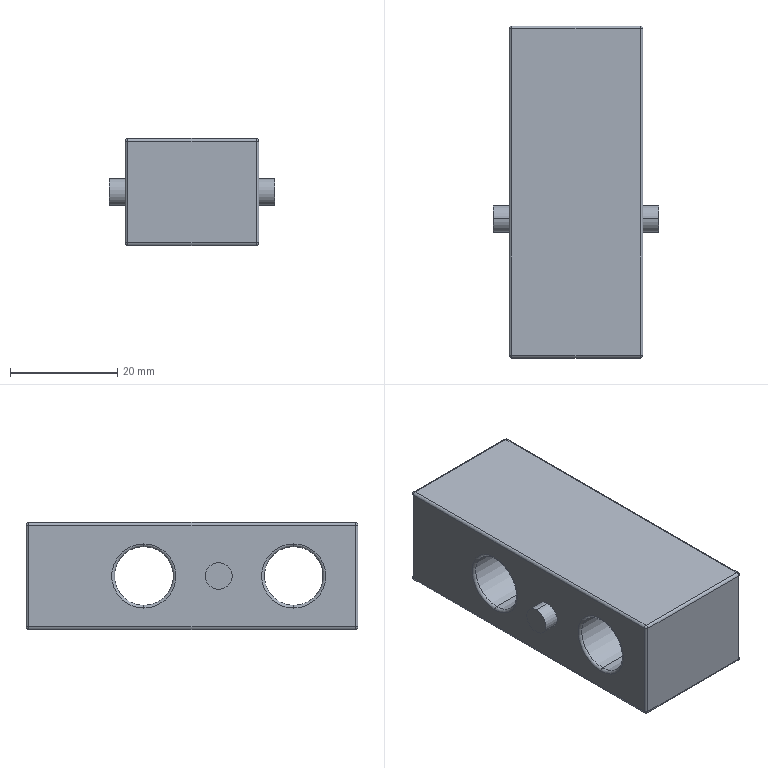Part | SolidWorks | features ICE 2, Extrusion 1, Fillet 1 | 1 solid | 49 faces | box 31 x 62 x 20 mm | volume 24637 mm3 | cylinder 22 | torus 10 | plane 9 | sphere 8 | commonest cylinder face diameters 1 x12 5 x4 11 x4 12 x2
STEP:
#1=CARTESIAN_POINT('',(12.5,-5.,-2.5));
#2=VERTEX_POINT('',#1);
#3=CARTESIAN_POINT('',(12.5,-5.,2.5));
#4=VERTEX_POINT('',#3);
#5=CARTESIAN_POINT('',(12.5,-5.,0.));
#6=DIRECTION('',(1.,0.,0.));
#7=DIRECTION('',(0.,0.,-1.));
#8=AXIS2_PLACEMENT_3D('',#5,#6,#7);
#9=CIRCLE('',#8,2.5);
#10=EDGE_CURVE('',#2,#4,#9,.T.);
#11=ORIENTED_EDGE('',*,*,#10,.T.);
#12=CARTESIAN_POINT('',(15.5,-5.,2.5));
#13=VERTEX_POINT('',#12);
#14=CARTESIAN_POINT('',(-25.571,-5.,2.5));
#15=DIRECTION('',(1.,0.,0.));
#16=VECTOR('',#15,1000.);
#17=LINE('',#14,#16);
#18=EDGE_CURVE('',#4,#13,#17,.T.);
#19=ORIENTED_EDGE('',*,*,#18,.T.);
#20=CARTESIAN_POINT('',(15.5,-5.,-2.5));
#21=VERTEX_POINT('',#20);
#22=CARTESIAN_POINT('',(15.5,-5.,0.));
#23=DIRECTION('',(1.,0.,0.));
#24=DIRECTION('',(0.,0.,-1.));
#25=AXIS2_PLACEMENT_3D('',#22,#23,#24);
#26=CIRCLE('',#25,2.5);
#27=EDGE_CURVE('',#21,#13,#26,.T.);
#28=ORIENTED_EDGE('',*,*,#27,.F.);
#29=CARTESIAN_POINT('',(-25.571,-5.,-2.5));
#30=DIRECTION('',(1.,0.,0.));
#31=VECTOR('',#30,1000.);
#32=LINE('',#29,#31);
#33=EDGE_CURVE('',#2,#21,#32,.T.);
#34=ORIENTED_EDGE('',*,*,#33,.F.);
#35=EDGE_LOOP('',(#11,#19,#28,#34));
#36=FACE_OUTER_BOUND('',#35,.T.);
#37=CARTESIAN_POINT('',(-25.571,-5.,0.));
#38=DIRECTION('',(1.,0.,0.));
#39=DIRECTION('',(0.,0.,-1.));
#40=AXIS2_PLACEMENT_3D('',#37,#38,#39);
#41=CYLINDRICAL_SURFACE('',#40,2.5);
#42=ADVANCED_FACE('',(#36),#41,.T.);
#43=CARTESIAN_POINT('',(-15.5,-5.,2.5));
#44=VERTEX_POINT('',#43);
#45=CARTESIAN_POINT('',(-15.5,-5.,-2.5));
#46=VERTEX_POINT('',#45);
#47=CARTESIAN_POINT('',(-15.5,-5.,0.));
#48=DIRECTION('',(-1.,0.,0.));
#49=DIRECTION('',(0.,0.,-1.));
#50=AXIS2_PLACEMENT_3D('',#47,#48,#49);
#51=CIRCLE('',#50,2.5);
#52=EDGE_CURVE('',#44,#46,#51,.T.);
#53=ORIENTED_EDGE('',*,*,#52,.F.);
#54=CARTESIAN_POINT('',(-12.5,-5.,2.5));
#55=VERTEX_POINT('',#54);
#56=CARTESIAN_POINT('',(-25.571,-5.,2.5));
#57=DIRECTION('',(1.,0.,0.));
#58=VECTOR('',#57,1000.);
#59=LINE('',#56,#58);
#60=EDGE_CURVE('',#44,#55,#59,.T.);
#61=ORIENTED_EDGE('',*,*,#60,.T.);
#62=CARTESIAN_POINT('',(-12.5,-5.,-2.5));
#63=VERTEX_POINT('',#62);
#64=CARTESIAN_POINT('',(-12.5,-5.,0.));
#65=DIRECTION('',(1.,0.,0.));
#66=DIRECTION('',(0.,0.,-1.));
#67=AXIS2_PLACEMENT_3D('',#64,#65,#66);
#68=CIRCLE('',#67,2.5);
#69=EDGE_CURVE('',#63,#55,#68,.T.);
#70=ORIENTED_EDGE('',*,*,#69,.F.);
#71=CARTESIAN_POINT('',(-25.571,-5.,-2.5));
#72=DIRECTION('',(1.,0.,0.));
#73=VECTOR('',#72,1000.);
#74=LINE('',#71,#73);
#75=EDGE_CURVE('',#46,#63,#74,.T.);
#76=ORIENTED_EDGE('',*,*,#75,.F.);
#77=EDGE_LOOP('',(#53,#61,#70,#76));
#78=FACE_OUTER_BOUND('',#77,.T.);
#79=CARTESIAN_POINT('',(-25.571,-5.,0.));
#80=DIRECTION('',(1.,0.,0.));
#81=DIRECTION('',(0.,0.,-1.));
#82=AXIS2_PLACEMENT_3D('',#79,#80,#81);
#83=CYLINDRICAL_SURFACE('',#82,2.5);
#84=ADVANCED_FACE('',(#78),#83,.T.);
#85=CARTESIAN_POINT('',(12.5,-19.,6.));
#86=VERTEX_POINT('',#85);
#87=CARTESIAN_POINT('',(12.5,-19.,-6.));
#88=VERTEX_POINT('',#87);
#89=CARTESIAN_POINT('',(12.5,-19.,0.));
#90=DIRECTION('',(-1.,0.,0.));
#91=DIRECTION('',(0.,0.,-1.));
#92=AXIS2_PLACEMENT_3D('',#89,#90,#91);
#93=CIRCLE('',#92,6.);
#94=EDGE_CURVE('',#86,#88,#93,.T.);
#95=ORIENTED_EDGE('',*,*,#94,.F.);
#96=CARTESIAN_POINT('',(12.,-19.,5.5));
#97=VERTEX_POINT('',#96);
#98=CARTESIAN_POINT('',(12.,-19.,6.));
#99=DIRECTION('',(0.,1.,0.));
#100=DIRECTION('',(0.,0.,1.));
#101=AXIS2_PLACEMENT_3D('',#98,#99,#100);
#102=CIRCLE('',#101,0.5);
#103=EDGE_CURVE('',#86,#97,#102,.T.);
#104=ORIENTED_EDGE('',*,*,#103,.T.);
#105=CARTESIAN_POINT('',(12.,-19.,-5.5));
#106=VERTEX_POINT('',#105);
#107=CARTESIAN_POINT('',(12.,-19.,0.));
#108=DIRECTION('',(1.,0.,0.));
#109=DIRECTION('',(0.,0.,-1.));
#110=AXIS2_PLACEMENT_3D('',#107,#108,#109);
#111=CIRCLE('',#110,5.5);
#112=EDGE_CURVE('',#106,#97,#111,.T.);
#113=ORIENTED_EDGE('',*,*,#112,.F.);
#114=CARTESIAN_POINT('',(12.,-19.,-6.));
#115=DIRECTION('',(0.,-1.,0.));
#116=DIRECTION('',(0.,0.,-1.));
#117=AXIS2_PLACEMENT_3D('',#114,#115,#116);
#118=CIRCLE('',#117,0.5);
#119=EDGE_CURVE('',#88,#106,#118,.T.);
#120=ORIENTED_EDGE('',*,*,#119,.F.);
#121=EDGE_LOOP('',(#95,#104,#113,#120));
#122=FACE_OUTER_BOUND('',#121,.T.);
#123=CARTESIAN_POINT('',(12.,-19.,0.));
#124=DIRECTION('',(1.,0.,0.));
#125=DIRECTION('',(0.,0.,-1.));
#126=AXIS2_PLACEMENT_3D('',#123,#124,#125);
#127=TOROIDAL_SURFACE('',#126,6.,0.5);
#128=ADVANCED_FACE('',(#122),#127,.T.);
#129=CARTESIAN_POINT('',(12.5,9.,6.));
#130=VERTEX_POINT('',#129);
#131=CARTESIAN_POINT('',(12.5,9.,-6.));
#132=VERTEX_POINT('',#131);
#133=CARTESIAN_POINT('',(12.5,9.,0.));
#134=DIRECTION('',(-1.,0.,0.));
#135=DIRECTION('',(0.,0.,-1.));
#136=AXIS2_PLACEMENT_3D('',#133,#134,#135);
#137=CIRCLE('',#136,6.);
#138=EDGE_CURVE('',#130,#132,#137,.T.);
#139=ORIENTED_EDGE('',*,*,#138,.F.);
#140=CARTESIAN_POINT('',(12.,9.,5.5));
#141=VERTEX_POINT('',#140);
#142=CARTESIAN_POINT('',(12.,9.,6.));
#143=DIRECTION('',(0.,1.,0.));
#144=DIRECTION('',(0.,0.,1.));
#145=AXIS2_PLACEMENT_3D('',#142,#143,#144);
#146=CIRCLE('',#145,0.5);
#147=EDGE_CURVE('',#130,#141,#146,.T.);
#148=ORIENTED_EDGE('',*,*,#147,.T.);
#149=CARTESIAN_POINT('',(12.,9.,-5.5));
#150=VERTEX_POINT('',#149);
#151=CARTESIAN_POINT('',(12.,9.,0.));
#152=DIRECTION('',(1.,0.,0.));
#153=DIRECTION('',(0.,0.,-1.));
#154=AXIS2_PLACEMENT_3D('',#151,#152,#153);
#155=CIRCLE('',#154,5.5);
#156=EDGE_CURVE('',#150,#141,#155,.T.);
#157=ORIENTED_EDGE('',*,*,#156,.F.);
#158=CARTESIAN_POINT('',(12.,9.,-6.));
#159=DIRECTION('',(0.,-1.,0.));
#160=DIRECTION('',(0.,0.,-1.));
#161=AXIS2_PLACEMENT_3D('',#158,#159,#160);
#162=CIRCLE('',#161,0.5);
#163=EDGE_CURVE('',#132,#150,#162,.T.);
#164=ORIENTED_EDGE('',*,*,#163,.F.);
#165=EDGE_LOOP('',(#139,#148,#157,#164));
#166=FACE_OUTER_BOUND('',#165,.T.);
#167=CARTESIAN_POINT('',(12.,9.,0.));
#168=DIRECTION('',(1.,0.,0.));
#169=DIRECTION('',(0.,0.,-1.));
#170=AXIS2_PLACEMENT_3D('',#167,#168,#169);
#171=TOROIDAL_SURFACE('',#170,6.,0.5);
#172=ADVANCED_FACE('',(#166),#171,.T.);
#173=CARTESIAN_POINT('',(-6.,24.,-9.5));
#174=VERTEX_POINT('',#173);
#175=CARTESIAN_POINT('',(6.,24.,-9.5));
#176=VERTEX_POINT('',#175);
#177=CARTESIAN_POINT('',(0.,24.,-9.5));
#178=DIRECTION('',(0.,0.,-1.));
#179=DIRECTION('',(1.,0.,0.));
#180=AXIS2_PLACEMENT_3D('',#177,#178,#179);
#181=CIRCLE('',#180,6.);
#182=EDGE_CURVE('',#174,#176,#181,.T.);
#183=ORIENTED_EDGE('',*,*,#182,.F.);
#184=CARTESIAN_POINT('',(-6.5,24.,-10.));
#185=VERTEX_POINT('',#184);
#186=CARTESIAN_POINT('',(-6.5,24.,-9.5));
#187=DIRECTION('',(0.,1.,0.));
#188=DIRECTION('',(-1.,0.,0.));
#189=AXIS2_PLACEMENT_3D('',#186,#187,#188);
#190=CIRCLE('',#189,0.5);
#191=EDGE_CURVE('',#174,#185,#190,.T.);
#192=ORIENTED_EDGE('',*,*,#191,.T.);
#193=CARTESIAN_POINT('',(0.,30.5,-10.));
#194=VERTEX_POINT('',#193);
#195=CARTESIAN_POINT('',(0.,24.,-10.));
#196=DIRECTION('',(0.,0.,1.));
#197=DIRECTION('',(1.,0.,0.));
#198=AXIS2_PLACEMENT_3D('',#195,#196,#197);
#199=CIRCLE('',#198,6.5);
#200=EDGE_CURVE('',#194,#185,#199,.T.);
#201=ORIENTED_EDGE('',*,*,#200,.F.);
#202=CARTESIAN_POINT('',(6.5,24.,-10.));
#203=VERTEX_POINT('',#202);
#204=CARTESIAN_POINT('',(0.,24.,-10.));
#205=DIRECTION('',(0.,0.,1.));
#206=DIRECTION('',(1.,0.,0.));
#207=AXIS2_PLACEMENT_3D('',#204,#205,#206);
#208=CIRCLE('',#207,6.5);
#209=EDGE_CURVE('',#203,#194,#208,.T.);
#210=ORIENTED_EDGE('',*,*,#209,.F.);
#211=CARTESIAN_POINT('',(6.5,24.,-9.5));
#212=DIRECTION('',(0.,-1.,0.));
#213=DIRECTION('',(0.,0.,-1.));
#214=AXIS2_PLACEMENT_3D('',#211,#212,#213);
#215=CIRCLE('',#214,0.5);
#216=EDGE_CURVE('',#176,#203,#215,.T.);
#217=ORIENTED_EDGE('',*,*,#216,.F.);
#218=EDGE_LOOP('',(#183,#192,#201,#210,#217));
#219=FACE_OUTER_BOUND('',#218,.T.);
#220=CARTESIAN_POINT('',(0.,24.,-9.5));
#221=DIRECTION('',(0.,0.,1.));
#222=DIRECTION('',(1.,0.,0.));
#223=AXIS2_PLACEMENT_3D('',#220,#221,#222);
#224=TOROIDAL_SURFACE('',#223,6.5,0.5);
#225=ADVANCED_FACE('',(#219),#224,.T.);
#226=CARTESIAN_POINT('',(-12.,-19.,5.5));
#227=VERTEX_POINT('',#226);
#228=CARTESIAN_POINT('',(-12.,-19.,-5.5));
#229=VERTEX_POINT('',#228);
#230=CARTESIAN_POINT('',(-12.,-19.,0.));
#231=DIRECTION('',(-1.,0.,0.));
#232=DIRECTION('',(0.,0.,-1.));
#233=AXIS2_PLACEMENT_3D('',#230,#231,#232);
#234=CIRCLE('',#233,5.5);
#235=EDGE_CURVE('',#227,#229,#234,.T.);
#236=ORIENTED_EDGE('',*,*,#235,.F.);
#237=CARTESIAN_POINT('',(-12.5,-19.,6.));
#238=VERTEX_POINT('',#237);
#239=CARTESIAN_POINT('',(-12.,-19.,6.));
#240=DIRECTION('',(0.,1.,0.));
#241=DIRECTION('',(0.,0.,1.));
#242=AXIS2_PLACEMENT_3D('',#239,#240,#241);
#243=CIRCLE('',#242,0.5);
#244=EDGE_CURVE('',#227,#238,#243,.T.);
#245=ORIENTED_EDGE('',*,*,#244,.T.);
#246=CARTESIAN_POINT('',(-12.5,-19.,-6.));
#247=VERTEX_POINT('',#246);
#248=CARTESIAN_POINT('',(-12.5,-19.,0.));
#249=DIRECTION('',(1.,0.,0.));
#250=DIRECTION('',(0.,0.,-1.));
#251=AXIS2_PLACEMENT_3D('',#248,#249,#250);
#252=CIRCLE('',#251,6.);
#253=EDGE_CURVE('',#247,#238,#252,.T.);
#254=ORIENTED_EDGE('',*,*,#253,.F.);
#255=CARTESIAN_POINT('',(-12.,-19.,-6.));
#256=DIRECTION('',(0.,-1.,0.));
#257=DIRECTION('',(0.,0.,-1.));
#258=AXIS2_PLACEMENT_3D('',#255,#256,#257);
#259=CIRCLE('',#258,0.5);
#260=EDGE_CURVE('',#229,#247,#259,.T.);
#261=ORIENTED_EDGE('',*,*,#260,.F.);
#262=EDGE_LOOP('',(#236,#245,#254,#261));
#263=FACE_OUTER_BOUND('',#262,.T.);
#264=CARTESIAN_POINT('',(-12.,-19.,0.));
#265=DIRECTION('',(1.,0.,0.));
#266=DIRECTION('',(0.,0.,-1.));
#267=AXIS2_PLACEMENT_3D('',#264,#265,#266);
#268=TOROIDAL_SURFACE('',#267,6.,0.5);
#269=ADVANCED_FACE('',(#263),#268,.T.);
#270=CARTESIAN_POINT('',(-12.,9.,5.5));
#271=VERTEX_POINT('',#270);
#272=CARTESIAN_POINT('',(-12.,9.,-5.5));
#273=VERTEX_POINT('',#272);
#274=CARTESIAN_POINT('',(-12.,9.,0.));
#275=DIRECTION('',(-1.,0.,0.));
#276=DIRECTION('',(0.,0.,-1.));
#277=AXIS2_PLACEMENT_3D('',#274,#275,#276);
#278=CIRCLE('',#277,5.5);
#279=EDGE_CURVE('',#271,#273,#278,.T.);
#280=ORIENTED_EDGE('',*,*,#279,.F.);
#281=CARTESIAN_POINT('',(-12.5,9.,6.));
#282=VERTEX_POINT('',#281);
#283=CARTESIAN_POINT('',(-12.,9.,6.));
#284=DIRECTION('',(0.,1.,0.));
#285=DIRECTION('',(0.,0.,1.));
#286=AXIS2_PLACEMENT_3D('',#283,#284,#285);
#287=CIRCLE('',#286,0.5);
#288=EDGE_CURVE('',#271,#282,#287,.T.);
#289=ORIENTED_EDGE('',*,*,#288,.T.);
#290=CARTESIAN_POINT('',(-12.5,9.,-6.));
#291=VERTEX_POINT('',#290);
#292=CARTESIAN_POINT('',(-12.5,9.,0.));
#293=DIRECTION('',(1.,0.,0.));
#294=DIRECTION('',(0.,0.,-1.));
#295=AXIS2_PLACEMENT_3D('',#292,#293,#294);
#296=CIRCLE('',#295,6.);
#297=EDGE_CURVE('',#291,#282,#296,.T.);
#298=ORIENTED_EDGE('',*,*,#297,.F.);
#299=CARTESIAN_POINT('',(-12.,9.,-6.));
#300=DIRECTION('',(0.,-1.,0.));
#301=DIRECTION('',(0.,0.,-1.));
#302=AXIS2_PLACEMENT_3D('',#299,#300,#301);
#303=CIRCLE('',#302,0.5);
#304=EDGE_CURVE('',#273,#291,#303,.T.);
#305=ORIENTED_EDGE('',*,*,#304,.F.);
#306=EDGE_LOOP('',(#280,#289,#298,#305));
#307=FACE_OUTER_BOUND('',#306,.T.);
#308=CARTESIAN_POINT('',(-12.,9.,0.));
#309=DIRECTION('',(1.,0.,0.));
#310=DIRECTION('',(0.,0.,-1.));
#311=AXIS2_PLACEMENT_3D('',#308,#309,#310);
#312=TOROIDAL_SURFACE('',#311,6.,0.5);
#313=ADVANCED_FACE('',(#307),#312,.T.);
#314=CARTESIAN_POINT('',(6.,24.,5.));
#315=VERTEX_POINT('',#314);
#316=CARTESIAN_POINT('',(-6.,24.,5.));
#317=VERTEX_POINT('',#316);
#318=CARTESIAN_POINT('',(0.,24.,5.));
#319=DIRECTION('',(0.,0.,-1.));
#320=DIRECTION('',(-1.,0.,0.));
#321=AXIS2_PLACEMENT_3D('',#318,#319,#320);
#322=CIRCLE('',#321,6.);
#323=EDGE_CURVE('',#315,#317,#322,.T.);
#324=ORIENTED_EDGE('',*,*,#323,.F.);
#325=CARTESIAN_POINT('',(6.,24.,5.));
#326=DIRECTION('',(0.,0.,-1.));
#327=VECTOR('',#326,1000.);
#328=LINE('',#325,#327);
#329=EDGE_CURVE('',#315,#176,#328,.T.);
#330=ORIENTED_EDGE('',*,*,#329,.T.);
#331=CARTESIAN_POINT('',(0.,24.,-9.5));
#332=DIRECTION('',(0.,0.,-1.));
#333=DIRECTION('',(1.,0.,0.));
#334=AXIS2_PLACEMENT_3D('',#331,#332,#333);
#335=CIRCLE('',#334,6.);
#336=EDGE_CURVE('',#176,#174,#335,.T.);
#337=ORIENTED_EDGE('',*,*,#336,.T.);
#338=CARTESIAN_POINT('',(-6.,24.,5.));
#339=DIRECTION('',(0.,0.,-1.));
#340=VECTOR('',#339,1000.);
#341=LINE('',#338,#340);
#342=EDGE_CURVE('',#317,#174,#341,.T.);
#343=ORIENTED_EDGE('',*,*,#342,.F.);
#344=EDGE_LOOP('',(#324,#330,#337,#343));
#345=FACE_OUTER_BOUND('',#344,.T.);
#346=CARTESIAN_POINT('',(0.,24.,5.));
#347=DIRECTION('',(0.,0.,-1.));
#348=DIRECTION('',(-1.,0.,0.));
#349=AXIS2_PLACEMENT_3D('',#346,#347,#348);
#350=CYLINDRICAL_SURFACE('',#349,6.);
#351=ADVANCED_FACE('',(#345),#350,.F.);
#352=CARTESIAN_POINT('',(12.,9.,0.));
#353=DIRECTION('',(1.,0.,0.));
#354=DIRECTION('',(0.,0.,-1.));
#355=AXIS2_PLACEMENT_3D('',#352,#353,#354);
#356=CIRCLE('',#355,5.5);
#357=EDGE_CURVE('',#141,#150,#356,.T.);
#358=ORIENTED_EDGE('',*,*,#357,.T.);
#359=CARTESIAN_POINT('',(12.5,9.,-5.5));
#360=DIRECTION('',(-1.,0.,0.));
#361=VECTOR('',#360,1000.);
#362=LINE('',#359,#361);
#363=EDGE_CURVE('',#150,#273,#362,.T.);
#364=ORIENTED_EDGE('',*,*,#363,.T.);
#365=CARTESIAN_POINT('',(-12.,9.,0.));
#366=DIRECTION('',(-1.,0.,0.));
#367=DIRECTION('',(0.,0.,-1.));
#368=AXIS2_PLACEMENT_3D('',#365,#366,#367);
#369=CIRCLE('',#368,5.5);
#370=EDGE_CURVE('',#273,#271,#369,.T.);
#371=ORIENTED_EDGE('',*,*,#370,.T.);
#372=CARTESIAN_POINT('',(12.5,9.,5.5));
#373=DIRECTION('',(-1.,0.,0.));
#374=VECTOR('',#373,1000.);
#375=LINE('',#372,#374);
#376=EDGE_CURVE('',#141,#271,#375,.T.);
#377=ORIENTED_EDGE('',*,*,#376,.F.);
#378=EDGE_LOOP('',(#358,#364,#371,#377));
#379=FACE_OUTER_BOUND('',#378,.T.);
#380=CARTESIAN_POINT('',(12.5,9.,0.));
#381=DIRECTION('',(-1.,0.,0.));
#382=DIRECTION('',(0.,0.,1.));
#383=AXIS2_PLACEMENT_3D('',#380,#381,#382);
#384=CYLINDRICAL_SURFACE('',#383,5.5);
#385=ADVANCED_FACE('',(#379),#384,.F.);
#386=CARTESIAN_POINT('',(12.,-19.,0.));
#387=DIRECTION('',(1.,0.,0.));
#388=DIRECTION('',(0.,0.,-1.));
#389=AXIS2_PLACEMENT_3D('',#386,#387,#388);
#390=CIRCLE('',#389,5.5);
#391=EDGE_CURVE('',#97,#106,#390,.T.);
#392=ORIENTED_EDGE('',*,*,#391,.T.);
#393=CARTESIAN_POINT('',(12.5,-19.,-5.5));
#394=DIRECTION('',(-1.,0.,0.));
#395=VECTOR('',#394,1000.);
#396=LINE('',#393,#395);
#397=EDGE_CURVE('',#106,#229,#396,.T.);
#398=ORIENTED_EDGE('',*,*,#397,.T.);
#399=CARTESIAN_POINT('',(-12.,-19.,0.));
#400=DIRECTION('',(-1.,0.,0.));
#401=DIRECTION('',(0.,0.,-1.));
#402=AXIS2_PLACEMENT_3D('',#399,#400,#401);
#403=CIRCLE('',#402,5.5);
#404=EDGE_CURVE('',#229,#227,#403,.T.);
#405=ORIENTED_EDGE('',*,*,#404,.T.);
#406=CARTESIAN_POINT('',(12.5,-19.,5.5));
#407=DIRECTION('',(-1.,0.,0.));
#408=VECTOR('',#407,1000.);
#409=LINE('',#406,#408);
#410=EDGE_CURVE('',#97,#227,#409,.T.);
#411=ORIENTED_EDGE('',*,*,#410,.F.);
#412=EDGE_LOOP('',(#392,#398,#405,#411));
#413=FACE_OUTER_BOUND('',#412,.T.);
#414=CARTESIAN_POINT('',(12.5,-19.,0.));
#415=DIRECTION('',(-1.,0.,0.));
#416=DIRECTION('',(0.,0.,1.));
#417=AXIS2_PLACEMENT_3D('',#414,#415,#416);
#418=CYLINDRICAL_SURFACE('',#417,5.5);
#419=ADVANCED_FACE('',(#413),#418,.F.);
#420=ORIENTED_EDGE('',*,*,#10,.F.);
#421=CARTESIAN_POINT('',(12.5,-5.,0.));
#422=DIRECTION('',(1.,0.,0.));
#423=DIRECTION('',(0.,0.,-1.));
#424=AXIS2_PLACEMENT_3D('',#421,#422,#423);
#425=CIRCLE('',#424,2.5);
#426=EDGE_CURVE('',#4,#2,#425,.T.);
#427=ORIENTED_EDGE('',*,*,#426,.F.);
#428=EDGE_LOOP('',(#420,#427));
#429=FACE_BOUND('',#428,.T.);
#430=CARTESIAN_POINT('',(12.5,9.,0.));
#431=DIRECTION('',(-1.,0.,0.));
#432=DIRECTION('',(0.,0.,-1.));
#433=AXIS2_PLACEMENT_3D('',#430,#431,#432);
#434=CIRCLE('',#433,6.);
#435=EDGE_CURVE('',#132,#130,#434,.T.);
#436=ORIENTED_EDGE('',*,*,#435,.T.);
#437=ORIENTED_EDGE('',*,*,#138,.T.);
#438=EDGE_LOOP('',(#436,#437));
#439=FACE_BOUND('',#438,.T.);
#440=CARTESIAN_POINT('',(12.5,-19.,0.));
#441=DIRECTION('',(-1.,0.,0.));
#442=DIRECTION('',(0.,0.,-1.));
#443=AXIS2_PLACEMENT_3D('',#440,#441,#442);
#444=CIRCLE('',#443,6.);
#445=EDGE_CURVE('',#88,#86,#444,.T.);
#446=ORIENTED_EDGE('',*,*,#445,.T.);
#447=ORIENTED_EDGE('',*,*,#94,.T.);
#448=EDGE_LOOP('',(#446,#447));
#449=FACE_BOUND('',#448,.T.);
#450=CARTESIAN_POINT('',(12.5,-30.5,9.5));
#451=VERTEX_POINT('',#450);
#452=CARTESIAN_POINT('',(12.5,-30.5,-9.5));
#453=VERTEX_POINT('',#452);
#454=CARTESIAN_POINT('',(12.5,-30.5,-10.));
#455=DIRECTION('',(0.,0.,-1.));
#456=VECTOR('',#455,1000.);
#457=LINE('',#454,#456);
#458=EDGE_CURVE('',#451,#453,#457,.T.);
#459=ORIENTED_EDGE('',*,*,#458,.T.);
#460=CARTESIAN_POINT('',(12.5,30.5,-9.5));
#461=VERTEX_POINT('',#460);
#462=CARTESIAN_POINT('',(12.5,31.,-9.5));
#463=DIRECTION('',(0.,1.,0.));
#464=VECTOR('',#463,1000.);
#465=LINE('',#462,#464);
#466=EDGE_CURVE('',#453,#461,#465,.T.);
#467=ORIENTED_EDGE('',*,*,#466,.T.);
#468=CARTESIAN_POINT('',(12.5,30.5,9.5));
#469=VERTEX_POINT('',#468);
#470=CARTESIAN_POINT('',(12.5,30.5,10.));
#471=DIRECTION('',(0.,0.,1.));
#472=VECTOR('',#471,1000.);
#473=LINE('',#470,#472);
#474=EDGE_CURVE('',#461,#469,#473,.T.);
#475=ORIENTED_EDGE('',*,*,#474,.T.);
#476=CARTESIAN_POINT('',(12.5,-31.,9.5));
#477=DIRECTION('',(0.,-1.,0.));
#478=VECTOR('',#477,1000.);
#479=LINE('',#476,#478);
#480=EDGE_CURVE('',#469,#451,#479,.T.);
#481=ORIENTED_EDGE('',*,*,#480,.T.);
#482=EDGE_LOOP('',(#459,#467,#475,#481));
#483=FACE_OUTER_BOUND('',#482,.T.);
#484=CARTESIAN_POINT('',(12.5,0.,0.));
#485=DIRECTION('',(1.,0.,0.));
#486=DIRECTION('',(0.,0.,-1.));
#487=AXIS2_PLACEMENT_3D('',#484,#485,#486);
#488=PLANE('',#487);
#489=ADVANCED_FACE('',(#429,#439,#449,#483),#488,.T.);
#490=ORIENTED_EDGE('',*,*,#69,.T.);
#491=CARTESIAN_POINT('',(-12.5,-5.,0.));
#492=DIRECTION('',(1.,0.,0.));
#493=DIRECTION('',(0.,0.,-1.));
#494=AXIS2_PLACEMENT_3D('',#491,#492,#493);
#495=CIRCLE('',#494,2.5);
#496=EDGE_CURVE('',#55,#63,#495,.T.);
#497=ORIENTED_EDGE('',*,*,#496,.T.);
#498=EDGE_LOOP('',(#490,#497));
#499=FACE_BOUND('',#498,.T.);
#500=ORIENTED_EDGE('',*,*,#297,.T.);
#501=CARTESIAN_POINT('',(-12.5,9.,0.));
#502=DIRECTION('',(1.,0.,0.));
#503=DIRECTION('',(0.,0.,-1.));
#504=AXIS2_PLACEMENT_3D('',#501,#502,#503);
#505=CIRCLE('',#504,6.);
#506=EDGE_CURVE('',#282,#291,#505,.T.);
#507=ORIENTED_EDGE('',*,*,#506,.T.);
#508=EDGE_LOOP('',(#500,#507));
#509=FACE_BOUND('',#508,.T.);
#510=ORIENTED_EDGE('',*,*,#253,.T.);
#511=CARTESIAN_POINT('',(-12.5,-19.,0.));
#512=DIRECTION('',(1.,0.,0.));
#513=DIRECTION('',(0.,0.,-1.));
#514=AXIS2_PLACEMENT_3D('',#511,#512,#513);
#515=CIRCLE('',#514,6.);
#516=EDGE_CURVE('',#238,#247,#515,.T.);
#517=ORIENTED_EDGE('',*,*,#516,.T.);
#518=EDGE_LOOP('',(#510,#517));
#519=FACE_BOUND('',#518,.T.);
#520=CARTESIAN_POINT('',(-12.5,30.5,-9.5));
#521=VERTEX_POINT('',#520);
#522=CARTESIAN_POINT('',(-12.5,-30.5,-9.5));
#523=VERTEX_POINT('',#522);
#524=CARTESIAN_POINT('',(-12.5,0.,-9.5));
#525=DIRECTION('',(0.,-1.,0.));
#526=VECTOR('',#525,1000.);
#527=LINE('',#524,#526);
#528=EDGE_CURVE('',#521,#523,#527,.T.);
#529=ORIENTED_EDGE('',*,*,#528,.T.);
#530=CARTESIAN_POINT('',(-12.5,-30.5,9.5));
#531=VERTEX_POINT('',#530);
#532=CARTESIAN_POINT('',(-12.5,-30.5,0.));
#533=DIRECTION('',(0.,0.,1.));
#534=VECTOR('',#533,1000.);
#535=LINE('',#532,#534);
#536=EDGE_CURVE('',#523,#531,#535,.T.);
#537=ORIENTED_EDGE('',*,*,#536,.T.);
#538=CARTESIAN_POINT('',(-12.5,30.5,9.5));
#539=VERTEX_POINT('',#538);
#540=CARTESIAN_POINT('',(-12.5,0.,9.5));
#541=DIRECTION('',(0.,1.,0.));
#542=VECTOR('',#541,1000.);
#543=LINE('',#540,#542);
#544=EDGE_CURVE('',#531,#539,#543,.T.);
#545=ORIENTED_EDGE('',*,*,#544,.T.);
#546=CARTESIAN_POINT('',(-12.5,30.5,0.));
#547=DIRECTION('',(0.,0.,-1.));
#548=VECTOR('',#547,1000.);
#549=LINE('',#546,#548);
#550=EDGE_CURVE('',#539,#521,#549,.T.);
#551=ORIENTED_EDGE('',*,*,#550,.T.);
#552=EDGE_LOOP('',(#529,#537,#545,#551));
#553=FACE_OUTER_BOUND('',#552,.T.);
#554=CARTESIAN_POINT('',(-12.5,0.,0.));
#555=DIRECTION('',(1.,0.,0.));
#556=DIRECTION('',(0.,0.,-1.));
#557=AXIS2_PLACEMENT_3D('',#554,#555,#556);
#558=PLANE('',#557);
#559=ADVANCED_FACE('',(#499,#509,#519,#553),#558,.F.);
#560=CARTESIAN_POINT('',(-12.,30.5,10.));
#561=VERTEX_POINT('',#560);
#562=CARTESIAN_POINT('',(-12.,-30.5,10.));
#563=VERTEX_POINT('',#562);
#564=CARTESIAN_POINT('',(-12.,-31.,10.));
#565=DIRECTION('',(0.,-1.,0.));
#566=VECTOR('',#565,1000.);
#567=LINE('',#564,#566);
#568=EDGE_CURVE('',#561,#563,#567,.T.);
#569=ORIENTED_EDGE('',*,*,#568,.T.);
#570=CARTESIAN_POINT('',(12.,-30.5,10.));
#571=VERTEX_POINT('',#570);
#572=CARTESIAN_POINT('',(12.5,-30.5,10.));
#573=DIRECTION('',(1.,0.,0.));
#574=VECTOR('',#573,1000.);
#575=LINE('',#572,#574);
#576=EDGE_CURVE('',#563,#571,#575,.T.);
#577=ORIENTED_EDGE('',*,*,#576,.T.);
#578=CARTESIAN_POINT('',(12.,30.5,10.));
#579=VERTEX_POINT('',#578);
#580=CARTESIAN_POINT('',(12.,31.,10.));
#581=DIRECTION('',(0.,1.,0.));
#582=VECTOR('',#581,1000.);
#583=LINE('',#580,#582);
#584=EDGE_CURVE('',#571,#579,#583,.T.);
#585=ORIENTED_EDGE('',*,*,#584,.T.);
#586=CARTESIAN_POINT('',(12.5,30.5,10.));
#587=DIRECTION('',(-1.,0.,0.));
#588=VECTOR('',#587,1000.);
#589=LINE('',#586,#588);
#590=EDGE_CURVE('',#579,#561,#589,.T.);
#591=ORIENTED_EDGE('',*,*,#590,.T.);
#592=EDGE_LOOP('',(#569,#577,#585,#591));
#593=FACE_OUTER_BOUND('',#592,.T.);
#594=CARTESIAN_POINT('',(12.5,-31.,10.));
#595=DIRECTION('',(0.,0.,-1.));
#596=DIRECTION('',(-1.,0.,0.));
#597=AXIS2_PLACEMENT_3D('',#594,#595,#596);
#598=PLANE('',#597);
#599=ADVANCED_FACE('',(#593),#598,.F.);
#600=CARTESIAN_POINT('',(12.,-31.,-9.5));
#601=VERTEX_POINT('',#600);
#602=CARTESIAN_POINT('',(12.,-31.,9.5));
#603=VERTEX_POINT('',#602);
#604=CARTESIAN_POINT('',(12.,-31.,10.));
#605=DIRECTION('',(0.,0.,1.));
#606=VECTOR('',#605,1000.);
#607=LINE('',#604,#606);
#608=EDGE_CURVE('',#601,#603,#607,.T.);
#609=ORIENTED_EDGE('',*,*,#608,.T.);
#610=CARTESIAN_POINT('',(-12.,-31.,9.5));
#611=VERTEX_POINT('',#610);
#612=CARTESIAN_POINT('',(12.5,-31.,9.5));
#613=DIRECTION('',(-1.,0.,0.));
#614=VECTOR('',#613,1000.);
#615=LINE('',#612,#614);
#616=EDGE_CURVE('',#603,#611,#615,.T.);
#617=ORIENTED_EDGE('',*,*,#616,.T.);
#618=CARTESIAN_POINT('',(-12.,-31.,-9.5));
#619=VERTEX_POINT('',#618);
#620=CARTESIAN_POINT('',(-12.,-31.,-10.));
#621=DIRECTION('',(0.,0.,-1.));
#622=VECTOR('',#621,1000.);
#623=LINE('',#620,#622);
#624=EDGE_CURVE('',#611,#619,#623,.T.);
#625=ORIENTED_EDGE('',*,*,#624,.T.);
#626=CARTESIAN_POINT('',(12.5,-31.,-9.5));
#627=DIRECTION('',(1.,0.,0.));
#628=VECTOR('',#627,1000.);
#629=LINE('',#626,#628);
#630=EDGE_CURVE('',#619,#601,#629,.T.);
#631=ORIENTED_EDGE('',*,*,#630,.T.);
#632=EDGE_LOOP('',(#609,#617,#625,#631));
#633=FACE_OUTER_BOUND('',#632,.T.);
#634=CARTESIAN_POINT('',(12.5,-31.,-10.));
#635=DIRECTION('',(0.,1.,0.));
#636=DIRECTION('',(0.,0.,1.));
#637=AXIS2_PLACEMENT_3D('',#634,#635,#636);
#638=PLANE('',#637);
#639=ADVANCED_FACE('',(#633),#638,.F.);
#640=ORIENTED_EDGE('',*,*,#200,.T.);
#641=CARTESIAN_POINT('',(0.,24.,-10.));
#642=DIRECTION('',(0.,0.,1.));
#643=DIRECTION('',(1.,0.,0.));
#644=AXIS2_PLACEMENT_3D('',#641,#642,#643);
#645=CIRCLE('',#644,6.5);
#646=EDGE_CURVE('',#185,#203,#645,.T.);
#647=ORIENTED_EDGE('',*,*,#646,.T.);
#648=ORIENTED_EDGE('',*,*,#209,.T.);
#649=CARTESIAN_POINT('',(12.,30.5,-10.));
#650=VERTEX_POINT('',#649);
#651=CARTESIAN_POINT('',(12.5,30.5,-10.));
#652=DIRECTION('',(1.,0.,0.));
#653=VECTOR('',#652,1000.);
#654=LINE('',#651,#653);
#655=EDGE_CURVE('',#194,#650,#654,.T.);
#656=ORIENTED_EDGE('',*,*,#655,.T.);
#657=CARTESIAN_POINT('',(12.,-30.5,-10.));
#658=VERTEX_POINT('',#657);
#659=CARTESIAN_POINT('',(12.,-31.,-10.));
#660=DIRECTION('',(0.,-1.,0.));
#661=VECTOR('',#660,1000.);
#662=LINE('',#659,#661);
#663=EDGE_CURVE('',#650,#658,#662,.T.);
#664=ORIENTED_EDGE('',*,*,#663,.T.);
#665=CARTESIAN_POINT('',(-12.,-30.5,-10.));
#666=VERTEX_POINT('',#665);
#667=CARTESIAN_POINT('',(12.5,-30.5,-10.));
#668=DIRECTION('',(-1.,0.,0.));
#669=VECTOR('',#668,1000.);
#670=LINE('',#667,#669);
#671=EDGE_CURVE('',#658,#666,#670,.T.);
#672=ORIENTED_EDGE('',*,*,#671,.T.);
#673=CARTESIAN_POINT('',(-12.,30.5,-10.));
#674=VERTEX_POINT('',#673);
#675=CARTESIAN_POINT('',(-12.,-31.,-10.));
#676=DIRECTION('',(0.,1.,0.));
#677=VECTOR('',#676,1000.);
#678=LINE('',#675,#677);
#679=EDGE_CURVE('',#666,#674,#678,.T.);
#680=ORIENTED_EDGE('',*,*,#679,.T.);
#681=CARTESIAN_POINT('',(12.5,30.5,-10.));
#682=DIRECTION('',(1.,0.,0.));
#683=VECTOR('',#682,1000.);
#684=LINE('',#681,#683);
#685=EDGE_CURVE('',#674,#194,#684,.T.);
#686=ORIENTED_EDGE('',*,*,#685,.T.);
#687=EDGE_LOOP('',(#640,#647,#648,#656,#664,#672,#680,#686));
#688=FACE_OUTER_BOUND('',#687,.T.);
#689=CARTESIAN_POINT('',(12.5,-31.,-10.));
#690=DIRECTION('',(0.,0.,1.));
#691=DIRECTION('',(1.,0.,0.));
#692=AXIS2_PLACEMENT_3D('',#689,#690,#691);
#693=PLANE('',#692);
#694=ADVANCED_FACE('',(#688),#693,.F.);
#695=CARTESIAN_POINT('',(12.,31.,9.5));
#696=VERTEX_POINT('',#695);
#697=CARTESIAN_POINT('',(12.,31.,-9.5));
#698=VERTEX_POINT('',#697);
#699=CARTESIAN_POINT('',(12.,31.,-10.));
#700=DIRECTION('',(0.,0.,-1.));
#701=VECTOR('',#700,1000.);
#702=LINE('',#699,#701);
#703=EDGE_CURVE('',#696,#698,#702,.T.);
#704=ORIENTED_EDGE('',*,*,#703,.T.);
#705=CARTESIAN_POINT('',(-12.,31.,-9.5));
#706=VERTEX_POINT('',#705);
#707=CARTESIAN_POINT('',(12.5,31.,-9.5));
#708=DIRECTION('',(-1.,0.,0.));
#709=VECTOR('',#708,1000.);
#710=LINE('',#707,#709);
#711=EDGE_CURVE('',#698,#706,#710,.T.);
#712=ORIENTED_EDGE('',*,*,#711,.T.);
#713=CARTESIAN_POINT('',(-12.,31.,9.5));
#714=VERTEX_POINT('',#713);
#715=CARTESIAN_POINT('',(-12.,31.,-10.));
#716=DIRECTION('',(0.,0.,1.));
#717=VECTOR('',#716,1000.);
#718=LINE('',#715,#717);
#719=EDGE_CURVE('',#706,#714,#718,.T.);
#720=ORIENTED_EDGE('',*,*,#719,.T.);
#721=CARTESIAN_POINT('',(12.5,31.,9.5));
#722=DIRECTION('',(1.,0.,0.));
#723=VECTOR('',#722,1000.);
#724=LINE('',#721,#723);
#725=EDGE_CURVE('',#714,#696,#724,.T.);
#726=ORIENTED_EDGE('',*,*,#725,.T.);
#727=EDGE_LOOP('',(#704,#712,#720,#726));
#728=FACE_OUTER_BOUND('',#727,.T.);
#729=CARTESIAN_POINT('',(12.5,31.,-10.));
#730=DIRECTION('',(0.,-1.,0.));
#731=DIRECTION('',(0.,0.,-1.));
#732=AXIS2_PLACEMENT_3D('',#729,#730,#731);
#733=PLANE('',#732);
#734=ADVANCED_FACE('',(#728),#733,.F.);
#735=ORIENTED_EDGE('',*,*,#397,.F.);
#736=ORIENTED_EDGE('',*,*,#112,.T.);
#737=ORIENTED_EDGE('',*,*,#410,.T.);
#738=ORIENTED_EDGE('',*,*,#235,.T.);
#739=EDGE_LOOP('',(#735,#736,#737,#738));
#740=FACE_OUTER_BOUND('',#739,.T.);
#741=CARTESIAN_POINT('',(12.5,-19.,0.));
#742=DIRECTION('',(-1.,0.,0.));
#743=DIRECTION('',(0.,0.,1.));
#744=AXIS2_PLACEMENT_3D('',#741,#742,#743);
#745=CYLINDRICAL_SURFACE('',#744,5.5);
#746=ADVANCED_FACE('',(#740),#745,.F.);
#747=ORIENTED_EDGE('',*,*,#363,.F.);
#748=ORIENTED_EDGE('',*,*,#156,.T.);
#749=ORIENTED_EDGE('',*,*,#376,.T.);
#750=ORIENTED_EDGE('',*,*,#279,.T.);
#751=EDGE_LOOP('',(#747,#748,#749,#750));
#752=FACE_OUTER_BOUND('',#751,.T.);
#753=CARTESIAN_POINT('',(12.5,9.,0.));
#754=DIRECTION('',(-1.,0.,0.));
#755=DIRECTION('',(0.,0.,1.));
#756=AXIS2_PLACEMENT_3D('',#753,#754,#755);
#757=CYLINDRICAL_SURFACE('',#756,5.5);
#758=ADVANCED_FACE('',(#752),#757,.F.);
#759=ORIENTED_EDGE('',*,*,#329,.F.);
#760=CARTESIAN_POINT('',(0.,24.,5.));
#761=DIRECTION('',(0.,0.,-1.));
#762=DIRECTION('',(-1.,0.,0.));
#763=AXIS2_PLACEMENT_3D('',#760,#761,#762);
#764=CIRCLE('',#763,6.);
#765=EDGE_CURVE('',#317,#315,#764,.T.);
#766=ORIENTED_EDGE('',*,*,#765,.F.);
#767=ORIENTED_EDGE('',*,*,#342,.T.);
#768=ORIENTED_EDGE('',*,*,#182,.T.);
#769=EDGE_LOOP('',(#759,#766,#767,#768));
#770=FACE_OUTER_BOUND('',#769,.T.);
#771=CARTESIAN_POINT('',(0.,24.,5.));
#772=DIRECTION('',(0.,0.,-1.));
#773=DIRECTION('',(-1.,0.,0.));
#774=AXIS2_PLACEMENT_3D('',#771,#772,#773);
#775=CYLINDRICAL_SURFACE('',#774,6.);
#776=ADVANCED_FACE('',(#770),#775,.F.);
#777=ORIENTED_EDGE('',*,*,#765,.T.);
#778=ORIENTED_EDGE('',*,*,#323,.T.);
#779=EDGE_LOOP('',(#777,#778));
#780=FACE_OUTER_BOUND('',#779,.T.);
#781=CARTESIAN_POINT('',(0.,24.,5.));
#782=DIRECTION('',(0.,0.,-1.));
#783=DIRECTION('',(-1.,0.,0.));
#784=AXIS2_PLACEMENT_3D('',#781,#782,#783);
#785=PLANE('',#784);
#786=ADVANCED_FACE('',(#780),#785,.T.);
#787=CARTESIAN_POINT('',(12.,30.5,-9.5));
#788=DIRECTION('',(1.,0.,0.));
#789=DIRECTION('',(0.,0.,-1.));
#790=AXIS2_PLACEMENT_3D('',#787,#788,#789);
#791=CIRCLE('',#790,0.5);
#792=EDGE_CURVE('',#650,#698,#791,.T.);
#793=ORIENTED_EDGE('',*,*,#792,.F.);
#794=ORIENTED_EDGE('',*,*,#655,.F.);
#795=ORIENTED_EDGE('',*,*,#685,.F.);
#796=CARTESIAN_POINT('',(-12.,30.5,-9.5));
#797=DIRECTION('',(-1.,0.,0.));
#798=DIRECTION('',(0.,0.,1.));
#799=AXIS2_PLACEMENT_3D('',#796,#797,#798);
#800=CIRCLE('',#799,0.5);
#801=EDGE_CURVE('',#706,#674,#800,.T.);
#802=ORIENTED_EDGE('',*,*,#801,.F.);
#803=ORIENTED_EDGE('',*,*,#711,.F.);
#804=EDGE_LOOP('',(#793,#794,#795,#802,#803));
#805=FACE_OUTER_BOUND('',#804,.T.);
#806=CARTESIAN_POINT('',(12.5,30.5,-9.5));
#807=DIRECTION('',(-1.,0.,0.));
#808=DIRECTION('',(0.,0.,1.));
#809=AXIS2_PLACEMENT_3D('',#806,#807,#808);
#810=CYLINDRICAL_SURFACE('',#809,0.5);
#811=ADVANCED_FACE('',(#805),#810,.T.);
#812=CARTESIAN_POINT('',(12.,30.5,-9.5));
#813=DIRECTION('',(0.,-1.,0.));
#814=DIRECTION('',(0.,0.,1.));
#815=AXIS2_PLACEMENT_3D('',#812,#813,#814);
#816=CIRCLE('',#815,0.5);
#817=EDGE_CURVE('',#650,#461,#816,.T.);
#818=ORIENTED_EDGE('',*,*,#817,.F.);
#819=ORIENTED_EDGE('',*,*,#792,.T.);
#820=CARTESIAN_POINT('',(12.,30.5,-9.5));
#821=DIRECTION('',(0.,0.,1.));
#822=DIRECTION('',(-1.,0.,0.));
#823=AXIS2_PLACEMENT_3D('',#820,#821,#822);
#824=CIRCLE('',#823,0.5);
#825=EDGE_CURVE('',#461,#698,#824,.T.);
#826=ORIENTED_EDGE('',*,*,#825,.F.);
#827=EDGE_LOOP('',(#818,#819,#826));
#828=FACE_OUTER_BOUND('',#827,.T.);
#829=CARTESIAN_POINT('',(12.,30.5,-9.5));
#830=DIRECTION('',(0.,1.,0.));
#831=DIRECTION('',(1.,0.,0.));
#832=AXIS2_PLACEMENT_3D('',#829,#830,#831);
#833=SPHERICAL_SURFACE('',#832,0.5);
#834=ADVANCED_FACE('',(#828),#833,.T.);
#835=CARTESIAN_POINT('',(-12.,30.5,-9.5));
#836=DIRECTION('',(0.,0.,1.));
#837=DIRECTION('',(-1.,0.,0.));
#838=AXIS2_PLACEMENT_3D('',#835,#836,#837);
#839=CIRCLE('',#838,0.5);
#840=EDGE_CURVE('',#706,#521,#839,.T.);
#841=ORIENTED_EDGE('',*,*,#840,.F.);
#842=ORIENTED_EDGE('',*,*,#801,.T.);
#843=CARTESIAN_POINT('',(-12.,30.5,-9.5));
#844=DIRECTION('',(0.,-1.,0.));
#845=DIRECTION('',(0.,0.,1.));
#846=AXIS2_PLACEMENT_3D('',#843,#844,#845);
#847=CIRCLE('',#846,0.5);
#848=EDGE_CURVE('',#521,#674,#847,.T.);
#849=ORIENTED_EDGE('',*,*,#848,.F.);
#850=EDGE_LOOP('',(#841,#842,#849));
#851=FACE_OUTER_BOUND('',#850,.T.);
#852=CARTESIAN_POINT('',(-12.,30.5,-9.5));
#853=DIRECTION('',(0.,1.,0.));
#854=DIRECTION('',(1.,0.,0.));
#855=AXIS2_PLACEMENT_3D('',#852,#853,#854);
#856=SPHERICAL_SURFACE('',#855,0.5);
#857=ADVANCED_FACE('',(#851),#856,.T.);
#858=ORIENTED_EDGE('',*,*,#825,.T.);
#859=ORIENTED_EDGE('',*,*,#703,.F.);
#860=CARTESIAN_POINT('',(12.,30.5,9.5));
#861=DIRECTION('',(0.,0.,1.));
#862=DIRECTION('',(1.,0.,0.));
#863=AXIS2_PLACEMENT_3D('',#860,#861,#862);
#864=CIRCLE('',#863,0.5);
#865=EDGE_CURVE('',#469,#696,#864,.T.);
#866=ORIENTED_EDGE('',*,*,#865,.F.);
#867=ORIENTED_EDGE('',*,*,#474,.F.);
#868=EDGE_LOOP('',(#858,#859,#866,#867));
#869=FACE_OUTER_BOUND('',#868,.T.);
#870=CARTESIAN_POINT('',(12.,30.5,0.));
#871=DIRECTION('',(0.,0.,-1.));
#872=DIRECTION('',(-1.,0.,0.));
#873=AXIS2_PLACEMENT_3D('',#870,#871,#872);
#874=CYLINDRICAL_SURFACE('',#873,0.5);
#875=ADVANCED_FACE('',(#869),#874,.T.);
#876=ORIENTED_EDGE('',*,*,#817,.T.);
#877=ORIENTED_EDGE('',*,*,#466,.F.);
#878=CARTESIAN_POINT('',(12.,-30.5,-9.5));
#879=DIRECTION('',(0.,-1.,0.));
#880=DIRECTION('',(0.,0.,-1.));
#881=AXIS2_PLACEMENT_3D('',#878,#879,#880);
#882=CIRCLE('',#881,0.5);
#883=EDGE_CURVE('',#658,#453,#882,.T.);
#884=ORIENTED_EDGE('',*,*,#883,.F.);
#885=ORIENTED_EDGE('',*,*,#663,.F.);
#886=EDGE_LOOP('',(#876,#877,#884,#885));
#887=FACE_OUTER_BOUND('',#886,.T.);
#888=CARTESIAN_POINT('',(12.,0.,-9.5));
#889=DIRECTION('',(0.,-1.,0.));
#890=DIRECTION('',(0.,0.,-1.));
#891=AXIS2_PLACEMENT_3D('',#888,#889,#890);
#892=CYLINDRICAL_SURFACE('',#891,0.5);
#893=ADVANCED_FACE('',(#887),#892,.T.);
#894=CARTESIAN_POINT('',(-12.,-30.5,-9.5));
#895=DIRECTION('',(-1.,0.,0.));
#896=DIRECTION('',(0.,0.,1.));
#897=AXIS2_PLACEMENT_3D('',#894,#895,#896);
#898=CIRCLE('',#897,0.5);
#899=EDGE_CURVE('',#666,#619,#898,.T.);
#900=ORIENTED_EDGE('',*,*,#899,.F.);
#901=ORIENTED_EDGE('',*,*,#671,.F.);
#902=CARTESIAN_POINT('',(12.,-30.5,-9.5));
#903=DIRECTION('',(1.,0.,0.));
#904=DIRECTION('',(0.,0.,-1.));
#905=AXIS2_PLACEMENT_3D('',#902,#903,#904);
#906=CIRCLE('',#905,0.5);
#907=EDGE_CURVE('',#601,#658,#906,.T.);
#908=ORIENTED_EDGE('',*,*,#907,.F.);
#909=ORIENTED_EDGE('',*,*,#630,.F.);
#910=EDGE_LOOP('',(#900,#901,#908,#909));
#911=FACE_OUTER_BOUND('',#910,.T.);
#912=CARTESIAN_POINT('',(12.5,-30.5,-9.5));
#913=DIRECTION('',(-1.,0.,0.));
#914=DIRECTION('',(0.,0.,1.));
#915=AXIS2_PLACEMENT_3D('',#912,#913,#914);
#916=CYLINDRICAL_SURFACE('',#915,0.5);
#917=ADVANCED_FACE('',(#911),#916,.T.);
#918=ORIENTED_EDGE('',*,*,#848,.T.);
#919=ORIENTED_EDGE('',*,*,#679,.F.);
#920=CARTESIAN_POINT('',(-12.,-30.5,-9.5));
#921=DIRECTION('',(0.,-1.,0.));
#922=DIRECTION('',(0.,0.,-1.));
#923=AXIS2_PLACEMENT_3D('',#920,#921,#922);
#924=CIRCLE('',#923,0.5);
#925=EDGE_CURVE('',#523,#666,#924,.T.);
#926=ORIENTED_EDGE('',*,*,#925,.F.);
#927=ORIENTED_EDGE('',*,*,#528,.F.);
#928=EDGE_LOOP('',(#918,#919,#926,#927));
#929=FACE_OUTER_BOUND('',#928,.T.);
#930=CARTESIAN_POINT('',(-12.,-31.,-9.5));
#931=DIRECTION('',(0.,1.,0.));
#932=DIRECTION('',(0.,0.,1.));
#933=AXIS2_PLACEMENT_3D('',#930,#931,#932);
#934=CYLINDRICAL_SURFACE('',#933,0.5);
#935=ADVANCED_FACE('',(#929),#934,.T.);
#936=ORIENTED_EDGE('',*,*,#840,.T.);
#937=ORIENTED_EDGE('',*,*,#550,.F.);
#938=CARTESIAN_POINT('',(-12.,30.5,9.5));
#939=DIRECTION('',(0.,0.,1.));
#940=DIRECTION('',(1.,0.,0.));
#941=AXIS2_PLACEMENT_3D('',#938,#939,#940);
#942=CIRCLE('',#941,0.5);
#943=EDGE_CURVE('',#714,#539,#942,.T.);
#944=ORIENTED_EDGE('',*,*,#943,.F.);
#945=ORIENTED_EDGE('',*,*,#719,.F.);
#946=EDGE_LOOP('',(#936,#937,#944,#945));
#947=FACE_OUTER_BOUND('',#946,.T.);
#948=CARTESIAN_POINT('',(-12.,30.5,-10.));
#949=DIRECTION('',(0.,0.,1.));
#950=DIRECTION('',(1.,0.,0.));
#951=AXIS2_PLACEMENT_3D('',#948,#949,#950);
#952=CYLINDRICAL_SURFACE('',#951,0.5);
#953=ADVANCED_FACE('',(#947),#952,.T.);
#954=CARTESIAN_POINT('',(12.,30.5,9.5));
#955=DIRECTION('',(1.,0.,0.));
#956=DIRECTION('',(0.,0.,-1.));
#957=AXIS2_PLACEMENT_3D('',#954,#955,#956);
#958=CIRCLE('',#957,0.5);
#959=EDGE_CURVE('',#696,#579,#958,.T.);
#960=ORIENTED_EDGE('',*,*,#959,.F.);
#961=ORIENTED_EDGE('',*,*,#725,.F.);
#962=CARTESIAN_POINT('',(-12.,30.5,9.5));
#963=DIRECTION('',(-1.,0.,0.));
#964=DIRECTION('',(0.,0.,1.));
#965=AXIS2_PLACEMENT_3D('',#962,#963,#964);
#966=CIRCLE('',#965,0.5);
#967=EDGE_CURVE('',#561,#714,#966,.T.);
#968=ORIENTED_EDGE('',*,*,#967,.F.);
#969=ORIENTED_EDGE('',*,*,#590,.F.);
#970=EDGE_LOOP('',(#960,#961,#968,#969));
#971=FACE_OUTER_BOUND('',#970,.T.);
#972=CARTESIAN_POINT('',(12.5,30.5,9.5));
#973=DIRECTION('',(-1.,0.,0.));
#974=DIRECTION('',(0.,0.,1.));
#975=AXIS2_PLACEMENT_3D('',#972,#973,#974);
#976=CYLINDRICAL_SURFACE('',#975,0.5);
#977=ADVANCED_FACE('',(#971),#976,.T.);
#978=ORIENTED_EDGE('',*,*,#865,.T.);
#979=ORIENTED_EDGE('',*,*,#959,.T.);
#980=CARTESIAN_POINT('',(12.,30.5,9.5));
#981=DIRECTION('',(0.,-1.,0.));
#982=DIRECTION('',(0.,0.,1.));
#983=AXIS2_PLACEMENT_3D('',#980,#981,#982);
#984=CIRCLE('',#983,0.5);
#985=EDGE_CURVE('',#469,#579,#984,.T.);
#986=ORIENTED_EDGE('',*,*,#985,.F.);
#987=EDGE_LOOP('',(#978,#979,#986));
#988=FACE_OUTER_BOUND('',#987,.T.);
#989=CARTESIAN_POINT('',(12.,30.5,9.5));
#990=DIRECTION('',(0.,1.,0.));
#991=DIRECTION('',(1.,0.,0.));
#992=AXIS2_PLACEMENT_3D('',#989,#990,#991);
#993=SPHERICAL_SURFACE('',#992,0.5);
#994=ADVANCED_FACE('',(#988),#993,.T.);
#995=ORIENTED_EDGE('',*,*,#907,.T.);
#996=ORIENTED_EDGE('',*,*,#883,.T.);
#997=CARTESIAN_POINT('',(12.,-30.5,-9.5));
#998=DIRECTION('',(0.,0.,1.));
#999=DIRECTION('',(-1.,0.,0.));
#1000=AXIS2_PLACEMENT_3D('',#997,#998,#999);
#1001=CIRCLE('',#1000,0.5);
#1002=EDGE_CURVE('',#601,#453,#1001,.T.);
#1003=ORIENTED_EDGE('',*,*,#1002,.F.);
#1004=EDGE_LOOP('',(#995,#996,#1003));
#1005=FACE_OUTER_BOUND('',#1004,.T.);
#1006=CARTESIAN_POINT('',(12.,-30.5,-9.5));
#1007=DIRECTION('',(0.,1.,0.));
#1008=DIRECTION('',(1.,0.,0.));
#1009=AXIS2_PLACEMENT_3D('',#1006,#1007,#1008);
#1010=SPHERICAL_SURFACE('',#1009,0.5);
#1011=ADVANCED_FACE('',(#1005),#1010,.T.);
#1012=ORIENTED_EDGE('',*,*,#925,.T.);
#1013=ORIENTED_EDGE('',*,*,#899,.T.);
#1014=CARTESIAN_POINT('',(-12.,-30.5,-9.5));
#1015=DIRECTION('',(0.,0.,1.));
#1016=DIRECTION('',(-1.,0.,0.));
#1017=AXIS2_PLACEMENT_3D('',#1014,#1015,#1016);
#1018=CIRCLE('',#1017,0.5);
#1019=EDGE_CURVE('',#523,#619,#1018,.T.);
#1020=ORIENTED_EDGE('',*,*,#1019,.F.);
#1021=EDGE_LOOP('',(#1012,#1013,#1020));
#1022=FACE_OUTER_BOUND('',#1021,.T.);
#1023=CARTESIAN_POINT('',(-12.,-30.5,-9.5));
#1024=DIRECTION('',(0.,1.,0.));
#1025=DIRECTION('',(1.,0.,0.));
#1026=AXIS2_PLACEMENT_3D('',#1023,#1024,#1025);
#1027=SPHERICAL_SURFACE('',#1026,0.5);
#1028=ADVANCED_FACE('',(#1022),#1027,.T.);
#1029=ORIENTED_EDGE('',*,*,#967,.T.);
#1030=ORIENTED_EDGE('',*,*,#943,.T.);
#1031=CARTESIAN_POINT('',(-12.,30.5,9.5));
#1032=DIRECTION('',(0.,-1.,0.));
#1033=DIRECTION('',(0.,0.,1.));
#1034=AXIS2_PLACEMENT_3D('',#1031,#1032,#1033);
#1035=CIRCLE('',#1034,0.5);
#1036=EDGE_CURVE('',#561,#539,#1035,.T.);
#1037=ORIENTED_EDGE('',*,*,#1036,.F.);
#1038=EDGE_LOOP('',(#1029,#1030,#1037));
#1039=FACE_OUTER_BOUND('',#1038,.T.);
#1040=CARTESIAN_POINT('',(-12.,30.5,9.5));
#1041=DIRECTION('',(0.,1.,0.));
#1042=DIRECTION('',(1.,0.,0.));
#1043=AXIS2_PLACEMENT_3D('',#1040,#1041,#1042);
#1044=SPHERICAL_SURFACE('',#1043,0.5);
#1045=ADVANCED_FACE('',(#1039),#1044,.T.);
#1046=ORIENTED_EDGE('',*,*,#985,.T.);
#1047=ORIENTED_EDGE('',*,*,#584,.F.);
#1048=CARTESIAN_POINT('',(12.,-30.5,9.5));
#1049=DIRECTION('',(0.,-1.,0.));
#1050=DIRECTION('',(0.,0.,-1.));
#1051=AXIS2_PLACEMENT_3D('',#1048,#1049,#1050);
#1052=CIRCLE('',#1051,0.5);
#1053=EDGE_CURVE('',#451,#571,#1052,.T.);
#1054=ORIENTED_EDGE('',*,*,#1053,.F.);
#1055=ORIENTED_EDGE('',*,*,#480,.F.);
#1056=EDGE_LOOP('',(#1046,#1047,#1054,#1055));
#1057=FACE_OUTER_BOUND('',#1056,.T.);
#1058=CARTESIAN_POINT('',(12.,0.,9.5));
#1059=DIRECTION('',(0.,1.,0.));
#1060=DIRECTION('',(0.,0.,1.));
#1061=AXIS2_PLACEMENT_3D('',#1058,#1059,#1060);
#1062=CYLINDRICAL_SURFACE('',#1061,0.5);
#1063=ADVANCED_FACE('',(#1057),#1062,.T.);
#1064=ORIENTED_EDGE('',*,*,#1002,.T.);
#1065=ORIENTED_EDGE('',*,*,#458,.F.);
#1066=CARTESIAN_POINT('',(12.,-30.5,9.5));
#1067=DIRECTION('',(0.,0.,1.));
#1068=DIRECTION('',(1.,0.,0.));
#1069=AXIS2_PLACEMENT_3D('',#1066,#1067,#1068);
#1070=CIRCLE('',#1069,0.5);
#1071=EDGE_CURVE('',#603,#451,#1070,.T.);
#1072=ORIENTED_EDGE('',*,*,#1071,.F.);
#1073=ORIENTED_EDGE('',*,*,#608,.F.);
#1074=EDGE_LOOP('',(#1064,#1065,#1072,#1073));
#1075=FACE_OUTER_BOUND('',#1074,.T.);
#1076=CARTESIAN_POINT('',(12.,-30.5,0.));
#1077=DIRECTION('',(0.,0.,1.));
#1078=DIRECTION('',(1.,0.,0.));
#1079=AXIS2_PLACEMENT_3D('',#1076,#1077,#1078);
#1080=CYLINDRICAL_SURFACE('',#1079,0.5);
#1081=ADVANCED_FACE('',(#1075),#1080,.T.);
#1082=ORIENTED_EDGE('',*,*,#1019,.T.);
#1083=ORIENTED_EDGE('',*,*,#624,.F.);
#1084=CARTESIAN_POINT('',(-12.,-30.5,9.5));
#1085=DIRECTION('',(0.,0.,1.));
#1086=DIRECTION('',(1.,0.,0.));
#1087=AXIS2_PLACEMENT_3D('',#1084,#1085,#1086);
#1088=CIRCLE('',#1087,0.5);
#1089=EDGE_CURVE('',#531,#611,#1088,.T.);
#1090=ORIENTED_EDGE('',*,*,#1089,.F.);
#1091=ORIENTED_EDGE('',*,*,#536,.F.);
#1092=EDGE_LOOP('',(#1082,#1083,#1090,#1091));
#1093=FACE_OUTER_BOUND('',#1092,.T.);
#1094=CARTESIAN_POINT('',(-12.,-30.5,-10.));
#1095=DIRECTION('',(0.,0.,-1.));
#1096=DIRECTION('',(-1.,0.,0.));
#1097=AXIS2_PLACEMENT_3D('',#1094,#1095,#1096);
#1098=CYLINDRICAL_SURFACE('',#1097,0.5);
#1099=ADVANCED_FACE('',(#1093),#1098,.T.);
#1100=ORIENTED_EDGE('',*,*,#1036,.T.);
#1101=ORIENTED_EDGE('',*,*,#544,.F.);
#1102=CARTESIAN_POINT('',(-12.,-30.5,9.5));
#1103=DIRECTION('',(0.,-1.,0.));
#1104=DIRECTION('',(0.,0.,-1.));
#1105=AXIS2_PLACEMENT_3D('',#1102,#1103,#1104);
#1106=CIRCLE('',#1105,0.5);
#1107=EDGE_CURVE('',#563,#531,#1106,.T.);
#1108=ORIENTED_EDGE('',*,*,#1107,.F.);
#1109=ORIENTED_EDGE('',*,*,#568,.F.);
#1110=EDGE_LOOP('',(#1100,#1101,#1108,#1109));
#1111=FACE_OUTER_BOUND('',#1110,.T.);
#1112=CARTESIAN_POINT('',(-12.,-31.,9.5));
#1113=DIRECTION('',(0.,-1.,0.));
#1114=DIRECTION('',(0.,0.,-1.));
#1115=AXIS2_PLACEMENT_3D('',#1112,#1113,#1114);
#1116=CYLINDRICAL_SURFACE('',#1115,0.5);
#1117=ADVANCED_FACE('',(#1111),#1116,.T.);
#1118=ORIENTED_EDGE('',*,*,#1071,.T.);
#1119=ORIENTED_EDGE('',*,*,#1053,.T.);
#1120=CARTESIAN_POINT('',(12.,-30.5,9.5));
#1121=DIRECTION('',(-1.,0.,0.));
#1122=DIRECTION('',(0.,0.,-1.));
#1123=AXIS2_PLACEMENT_3D('',#1120,#1121,#1122);
#1124=CIRCLE('',#1123,0.5);
#1125=EDGE_CURVE('',#603,#571,#1124,.T.);
#1126=ORIENTED_EDGE('',*,*,#1125,.F.);
#1127=EDGE_LOOP('',(#1118,#1119,#1126));
#1128=FACE_OUTER_BOUND('',#1127,.T.);
#1129=CARTESIAN_POINT('',(12.,-30.5,9.5));
#1130=DIRECTION('',(0.,1.,0.));
#1131=DIRECTION('',(1.,0.,0.));
#1132=AXIS2_PLACEMENT_3D('',#1129,#1130,#1131);
#1133=SPHERICAL_SURFACE('',#1132,0.5);
#1134=ADVANCED_FACE('',(#1128),#1133,.T.);
#1135=ORIENTED_EDGE('',*,*,#1107,.T.);
#1136=ORIENTED_EDGE('',*,*,#1089,.T.);
#1137=CARTESIAN_POINT('',(-12.,-30.5,9.5));
#1138=DIRECTION('',(1.,0.,0.));
#1139=DIRECTION('',(0.,0.,1.));
#1140=AXIS2_PLACEMENT_3D('',#1137,#1138,#1139);
#1141=CIRCLE('',#1140,0.5);
#1142=EDGE_CURVE('',#563,#611,#1141,.T.);
#1143=ORIENTED_EDGE('',*,*,#1142,.F.);
#1144=EDGE_LOOP('',(#1135,#1136,#1143));
#1145=FACE_OUTER_BOUND('',#1144,.T.);
#1146=CARTESIAN_POINT('',(-12.,-30.5,9.5));
#1147=DIRECTION('',(0.,1.,0.));
#1148=DIRECTION('',(1.,0.,0.));
#1149=AXIS2_PLACEMENT_3D('',#1146,#1147,#1148);
#1150=SPHERICAL_SURFACE('',#1149,0.5);
#1151=ADVANCED_FACE('',(#1145),#1150,.T.);
#1152=ORIENTED_EDGE('',*,*,#1125,.T.);
#1153=ORIENTED_EDGE('',*,*,#576,.F.);
#1154=ORIENTED_EDGE('',*,*,#1142,.T.);
#1155=ORIENTED_EDGE('',*,*,#616,.F.);
#1156=EDGE_LOOP('',(#1152,#1153,#1154,#1155));
#1157=FACE_OUTER_BOUND('',#1156,.T.);
#1158=CARTESIAN_POINT('',(12.5,-30.5,9.5));
#1159=DIRECTION('',(-1.,0.,0.));
#1160=DIRECTION('',(0.,0.,1.));
#1161=AXIS2_PLACEMENT_3D('',#1158,#1159,#1160);
#1162=CYLINDRICAL_SURFACE('',#1161,0.5);
#1163=ADVANCED_FACE('',(#1157),#1162,.T.);
#1164=ORIENTED_EDGE('',*,*,#288,.F.);
#1165=ORIENTED_EDGE('',*,*,#370,.F.);
#1166=ORIENTED_EDGE('',*,*,#304,.T.);
#1167=ORIENTED_EDGE('',*,*,#506,.F.);
#1168=EDGE_LOOP('',(#1164,#1165,#1166,#1167));
#1169=FACE_OUTER_BOUND('',#1168,.T.);
#1170=CARTESIAN_POINT('',(-12.,9.,0.));
#1171=DIRECTION('',(1.,0.,0.));
#1172=DIRECTION('',(0.,0.,-1.));
#1173=AXIS2_PLACEMENT_3D('',#1170,#1171,#1172);
#1174=TOROIDAL_SURFACE('',#1173,6.,0.5);
#1175=ADVANCED_FACE('',(#1169),#1174,.T.);
#1176=ORIENTED_EDGE('',*,*,#244,.F.);
#1177=ORIENTED_EDGE('',*,*,#404,.F.);
#1178=ORIENTED_EDGE('',*,*,#260,.T.);
#1179=ORIENTED_EDGE('',*,*,#516,.F.);
#1180=EDGE_LOOP('',(#1176,#1177,#1178,#1179));
#1181=FACE_OUTER_BOUND('',#1180,.T.);
#1182=CARTESIAN_POINT('',(-12.,-19.,0.));
#1183=DIRECTION('',(1.,0.,0.));
#1184=DIRECTION('',(0.,0.,-1.));
#1185=AXIS2_PLACEMENT_3D('',#1182,#1183,#1184);
#1186=TOROIDAL_SURFACE('',#1185,6.,0.5);
#1187=ADVANCED_FACE('',(#1181),#1186,.T.);
#1188=ORIENTED_EDGE('',*,*,#191,.F.);
#1189=ORIENTED_EDGE('',*,*,#336,.F.);
#1190=ORIENTED_EDGE('',*,*,#216,.T.);
#1191=ORIENTED_EDGE('',*,*,#646,.F.);
#1192=EDGE_LOOP('',(#1188,#1189,#1190,#1191));
#1193=FACE_OUTER_BOUND('',#1192,.T.);
#1194=CARTESIAN_POINT('',(0.,24.,-9.5));
#1195=DIRECTION('',(0.,0.,1.));
#1196=DIRECTION('',(1.,0.,0.));
#1197=AXIS2_PLACEMENT_3D('',#1194,#1195,#1196);
#1198=TOROIDAL_SURFACE('',#1197,6.5,0.5);
#1199=ADVANCED_FACE('',(#1193),#1198,.T.);
#1200=ORIENTED_EDGE('',*,*,#147,.F.);
#1201=ORIENTED_EDGE('',*,*,#435,.F.);
#1202=ORIENTED_EDGE('',*,*,#163,.T.);
#1203=ORIENTED_EDGE('',*,*,#357,.F.);
#1204=EDGE_LOOP('',(#1200,#1201,#1202,#1203));
#1205=FACE_OUTER_BOUND('',#1204,.T.);
#1206=CARTESIAN_POINT('',(12.,9.,0.));
#1207=DIRECTION('',(1.,0.,0.));
#1208=DIRECTION('',(0.,0.,-1.));
#1209=AXIS2_PLACEMENT_3D('',#1206,#1207,#1208);
#1210=TOROIDAL_SURFACE('',#1209,6.,0.5);
#1211=ADVANCED_FACE('',(#1205),#1210,.T.);
#1212=ORIENTED_EDGE('',*,*,#103,.F.);
#1213=ORIENTED_EDGE('',*,*,#445,.F.);
#1214=ORIENTED_EDGE('',*,*,#119,.T.);
#1215=ORIENTED_EDGE('',*,*,#391,.F.);
#1216=EDGE_LOOP('',(#1212,#1213,#1214,#1215));
#1217=FACE_OUTER_BOUND('',#1216,.T.);
#1218=CARTESIAN_POINT('',(12.,-19.,0.));
#1219=DIRECTION('',(1.,0.,0.));
#1220=DIRECTION('',(0.,0.,-1.));
#1221=AXIS2_PLACEMENT_3D('',#1218,#1219,#1220);
#1222=TOROIDAL_SURFACE('',#1221,6.,0.5);
#1223=ADVANCED_FACE('',(#1217),#1222,.T.);
#1224=CARTESIAN_POINT('',(-15.5,-5.,0.));
#1225=DIRECTION('',(-1.,0.,0.));
#1226=DIRECTION('',(0.,0.,-1.));
#1227=AXIS2_PLACEMENT_3D('',#1224,#1225,#1226);
#1228=CIRCLE('',#1227,2.5);
#1229=EDGE_CURVE('',#46,#44,#1228,.T.);
#1230=ORIENTED_EDGE('',*,*,#1229,.T.);
#1231=ORIENTED_EDGE('',*,*,#52,.T.);
#1232=EDGE_LOOP('',(#1230,#1231));
#1233=FACE_OUTER_BOUND('',#1232,.T.);
#1234=CARTESIAN_POINT('',(-15.5,0.,0.));
#1235=DIRECTION('',(1.,0.,0.));
#1236=DIRECTION('',(0.,0.,-1.));
#1237=AXIS2_PLACEMENT_3D('',#1234,#1235,#1236);
#1238=PLANE('',#1237);
#1239=ADVANCED_FACE('',(#1233),#1238,.F.);
#1240=ORIENTED_EDGE('',*,*,#60,.F.);
#1241=ORIENTED_EDGE('',*,*,#1229,.F.);
#1242=ORIENTED_EDGE('',*,*,#75,.T.);
#1243=ORIENTED_EDGE('',*,*,#496,.F.);
#1244=EDGE_LOOP('',(#1240,#1241,#1242,#1243));
#1245=FACE_OUTER_BOUND('',#1244,.T.);
#1246=CARTESIAN_POINT('',(-25.571,-5.,0.));
#1247=DIRECTION('',(1.,0.,0.));
#1248=DIRECTION('',(0.,0.,-1.));
#1249=AXIS2_PLACEMENT_3D('',#1246,#1247,#1248);
#1250=CYLINDRICAL_SURFACE('',#1249,2.5);
#1251=ADVANCED_FACE('',(#1245),#1250,.T.);
#1252=ORIENTED_EDGE('',*,*,#18,.F.);
#1253=ORIENTED_EDGE('',*,*,#426,.T.);
#1254=ORIENTED_EDGE('',*,*,#33,.T.);
#1255=CARTESIAN_POINT('',(15.5,-5.,0.));
#1256=DIRECTION('',(1.,0.,0.));
#1257=DIRECTION('',(0.,0.,-1.));
#1258=AXIS2_PLACEMENT_3D('',#1255,#1256,#1257);
#1259=CIRCLE('',#1258,2.5);
#1260=EDGE_CURVE('',#13,#21,#1259,.T.);
#1261=ORIENTED_EDGE('',*,*,#1260,.F.);
#1262=EDGE_LOOP('',(#1252,#1253,#1254,#1261));
#1263=FACE_OUTER_BOUND('',#1262,.T.);
#1264=CARTESIAN_POINT('',(-25.571,-5.,0.));
#1265=DIRECTION('',(1.,0.,0.));
#1266=DIRECTION('',(0.,0.,-1.));
#1267=AXIS2_PLACEMENT_3D('',#1264,#1265,#1266);
#1268=CYLINDRICAL_SURFACE('',#1267,2.5);
#1269=ADVANCED_FACE('',(#1263),#1268,.T.);
#1270=ORIENTED_EDGE('',*,*,#27,.T.);
#1271=ORIENTED_EDGE('',*,*,#1260,.T.);
#1272=EDGE_LOOP('',(#1270,#1271));
#1273=FACE_OUTER_BOUND('',#1272,.T.);
#1274=CARTESIAN_POINT('',(15.5,-5.,0.));
#1275=DIRECTION('',(1.,0.,0.));
#1276=DIRECTION('',(0.,0.,-1.));
#1277=AXIS2_PLACEMENT_3D('',#1274,#1275,#1276);
#1278=PLANE('',#1277);
#1279=ADVANCED_FACE('',(#1273),#1278,.T.);
#1280=CLOSED_SHELL('',(#42,#84,#128,#172,#225,#269,#313,#351,#385,#419,#489,#559,#599,#639,#694,#734,#746,#758,#776,#786,#811,#834,#857,#875,#893,#917,#935,#953,#977,#994,#1011,#1028,#1045,#1063,#1081,#1099,#1117,#1134,#1151,#1163,#1175,#1187,#1199,#1211,#1223,#1239,#1251,#1269,#1279));
#1281=MANIFOLD_SOLID_BREP('',#1280);
#1282=CARTESIAN_POINT('',(0.,0.,0.));
#1283=DIRECTION('',(0.,0.,1.));
#1284=DIRECTION('',(1.,0.,0.));
#1285=AXIS2_PLACEMENT_3D('',#1282,#1283,#1284);
#1286=(LENGTH_UNIT()NAMED_UNIT(*)SI_UNIT(.MILLI.,.METRE.));
#1287=UNCERTAINTY_MEASURE_WITH_UNIT(LENGTH_MEASURE(0.00001),#1286,'','');
#1288=(NAMED_UNIT(*)PLANE_ANGLE_UNIT()SI_UNIT($,.RADIAN.));
#1289=(NAMED_UNIT(*)SI_UNIT($,.STERADIAN.)SOLID_ANGLE_UNIT());
#1290=(GEOMETRIC_REPRESENTATION_CONTEXT(3)GLOBAL_UNCERTAINTY_ASSIGNED_CONTEXT((#1287))GLOBAL_UNIT_ASSIGNED_CONTEXT((#1286,#1288,#1289))REPRESENTATION_CONTEXT('',''));
#1291=ADVANCED_BREP_SHAPE_REPRESENTATION('',(#1281,#1285),#1290);